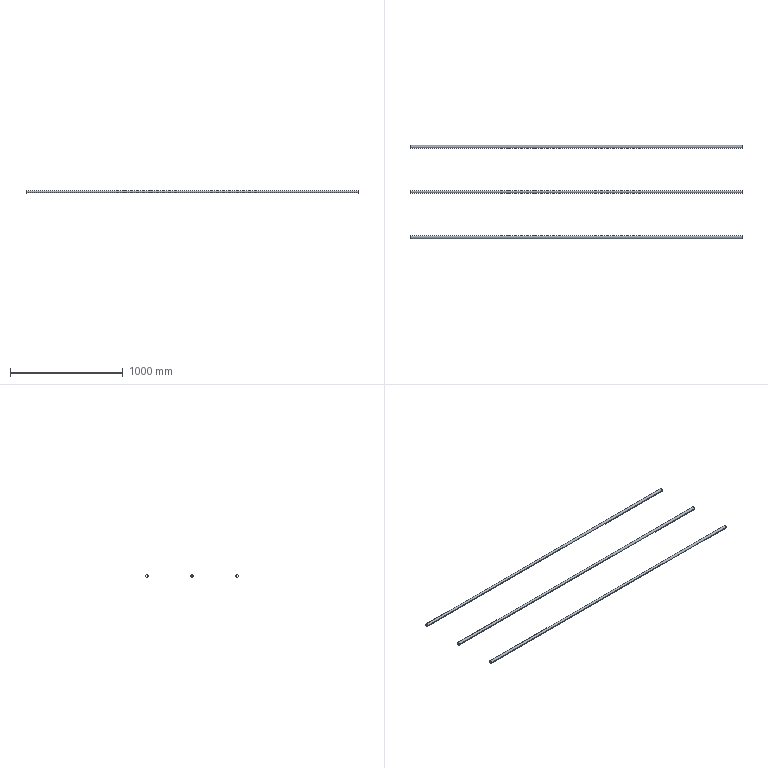Part | STEP file | E3-中转釜护栏1栏杆_Default<As Machined> | 3 solids | 18 faces | box 2940 x 825 x 25 mm | volume 976737 mm3 | cylinder 12 | plane 6 | commonest cylinder face diameters 22 x6 25 x6
STEP:
#1=CARTESIAN_POINT('',(0.,0.,0.));
#2=DIRECTION('',(0.,0.,1.));
#3=DIRECTION('',(1.,0.,0.));
#4=AXIS2_PLACEMENT_3D('',#1,#2,#3);
#5=CARTESIAN_POINT('',(1470.,787.5,0.));
#6=VERTEX_POINT('',#5);
#7=CARTESIAN_POINT('',(1470.,812.5,0.));
#8=VERTEX_POINT('',#7);
#9=CARTESIAN_POINT('',(1470.,800.,0.));
#10=DIRECTION('',(-1.,0.,0.));
#11=DIRECTION('',(0.,1.,0.));
#12=AXIS2_PLACEMENT_3D('',#9,#10,#11);
#13=CIRCLE('',#12,12.5);
#14=CARTESIAN_POINT('',(1470.,800.,0.));
#15=DIRECTION('',(-1.,0.,0.));
#16=DIRECTION('',(0.,-1.,0.));
#17=AXIS2_PLACEMENT_3D('',#14,#15,#16);
#18=CYLINDRICAL_SURFACE('',#17,12.5);
#19=CARTESIAN_POINT('',(-3.142,0.));
#20=DIRECTION('',(1.,0.));
#21=VECTOR('',#20,1.);
#22=LINE('',#19,#21);
#23=(GEOMETRIC_REPRESENTATION_CONTEXT(2)PARAMETRIC_REPRESENTATION_CONTEXT()REPRESENTATION_CONTEXT('',''));
#24=DEFINITIONAL_REPRESENTATION('',(#22),#23);
#25=PCURVE('',#18,#24);
#26=CARTESIAN_POINT('',(1470.,800.,0.));
#27=DIRECTION('',(1.,0.,0.));
#28=DIRECTION('',(0.,1.,0.));
#29=AXIS2_PLACEMENT_3D('',#26,#27,#28);
#30=PLANE('',#29);
#31=CARTESIAN_POINT('',(12.5,0.));
#32=CARTESIAN_POINT('',(12.5,-21.651));
#33=CARTESIAN_POINT('',(-6.25,-10.825));
#34=CARTESIAN_POINT('',(-25.,0.));
#35=CARTESIAN_POINT('',(-6.25,10.825));
#36=CARTESIAN_POINT('',(12.5,21.651));
#37=CARTESIAN_POINT('',(12.5,0.));
#38=(BOUNDED_CURVE()B_SPLINE_CURVE(2,(#31,#32,#33,#34,#35,#36,#37),.UNSPECIFIED.,.T.,.F.)B_SPLINE_CURVE_WITH_KNOTS((1,2,2,2,2,1),(-2.094,0.,2.094,4.189,6.283,8.378),.UNSPECIFIED.)CURVE()GEOMETRIC_REPRESENTATION_ITEM()RATIONAL_B_SPLINE_CURVE((1.,0.5,1.,0.5,1.,0.5,1.))REPRESENTATION_ITEM(''));
#39=(GEOMETRIC_REPRESENTATION_CONTEXT(2)PARAMETRIC_REPRESENTATION_CONTEXT()REPRESENTATION_CONTEXT('',''));
#40=DEFINITIONAL_REPRESENTATION('',(#38),#39);
#41=PCURVE('',#30,#40);
#42=SURFACE_CURVE('',#13,(#25,#41),.PCURVE_S1.);
#43=EDGE_CURVE('',#6,#8,#42,.T.);
#44=ORIENTED_EDGE('',*,*,#43,.T.);
#45=CARTESIAN_POINT('',(-1470.,812.5,0.));
#46=VERTEX_POINT('',#45);
#47=CARTESIAN_POINT('',(1470.,812.5,0.));
#48=DIRECTION('',(-1.,0.,0.));
#49=VECTOR('',#48,1.);
#50=LINE('',#47,#49);
#51=CARTESIAN_POINT('',(3.142,0.));
#52=DIRECTION('',(0.,1.));
#53=VECTOR('',#52,1.);
#54=LINE('',#51,#53);
#55=(GEOMETRIC_REPRESENTATION_CONTEXT(2)PARAMETRIC_REPRESENTATION_CONTEXT()REPRESENTATION_CONTEXT('',''));
#56=DEFINITIONAL_REPRESENTATION('',(#54),#55);
#57=PCURVE('',#18,#56);
#58=CARTESIAN_POINT('',(1470.,800.,0.));
#59=DIRECTION('',(-1.,0.,0.));
#60=DIRECTION('',(0.,-1.,0.));
#61=AXIS2_PLACEMENT_3D('',#58,#59,#60);
#62=CYLINDRICAL_SURFACE('',#61,12.5);
#63=CARTESIAN_POINT('',(3.142,0.));
#64=DIRECTION('',(0.,1.));
#65=VECTOR('',#64,1.);
#66=LINE('',#63,#65);
#67=(GEOMETRIC_REPRESENTATION_CONTEXT(2)PARAMETRIC_REPRESENTATION_CONTEXT()REPRESENTATION_CONTEXT('',''));
#68=DEFINITIONAL_REPRESENTATION('',(#66),#67);
#69=PCURVE('',#62,#68);
#70=SURFACE_CURVE('',#50,(#57,#69),.PCURVE_S1.);
#71=EDGE_CURVE('',#8,#46,#70,.T.);
#72=ORIENTED_EDGE('',*,*,#71,.T.);
#73=CARTESIAN_POINT('',(-1470.,787.5,0.));
#74=VERTEX_POINT('',#73);
#75=CARTESIAN_POINT('',(-1470.,800.,0.));
#76=DIRECTION('',(-1.,0.,0.));
#77=DIRECTION('',(0.,1.,0.));
#78=AXIS2_PLACEMENT_3D('',#75,#76,#77);
#79=CIRCLE('',#78,12.5);
#80=CARTESIAN_POINT('',(-3.142,2940.));
#81=DIRECTION('',(1.,0.));
#82=VECTOR('',#81,1.);
#83=LINE('',#80,#82);
#84=(GEOMETRIC_REPRESENTATION_CONTEXT(2)PARAMETRIC_REPRESENTATION_CONTEXT()REPRESENTATION_CONTEXT('',''));
#85=DEFINITIONAL_REPRESENTATION('',(#83),#84);
#86=PCURVE('',#18,#85);
#87=CARTESIAN_POINT('',(-1470.,800.,0.));
#88=DIRECTION('',(1.,0.,0.));
#89=DIRECTION('',(0.,1.,0.));
#90=AXIS2_PLACEMENT_3D('',#87,#88,#89);
#91=PLANE('',#90);
#92=CARTESIAN_POINT('',(12.5,0.));
#93=CARTESIAN_POINT('',(12.5,-21.651));
#94=CARTESIAN_POINT('',(-6.25,-10.825));
#95=CARTESIAN_POINT('',(-25.,0.));
#96=CARTESIAN_POINT('',(-6.25,10.825));
#97=CARTESIAN_POINT('',(12.5,21.651));
#98=CARTESIAN_POINT('',(12.5,0.));
#99=(BOUNDED_CURVE()B_SPLINE_CURVE(2,(#92,#93,#94,#95,#96,#97,#98),.UNSPECIFIED.,.T.,.F.)B_SPLINE_CURVE_WITH_KNOTS((1,2,2,2,2,1),(-2.094,0.,2.094,4.189,6.283,8.378),.UNSPECIFIED.)CURVE()GEOMETRIC_REPRESENTATION_ITEM()RATIONAL_B_SPLINE_CURVE((1.,0.5,1.,0.5,1.,0.5,1.))REPRESENTATION_ITEM(''));
#100=(GEOMETRIC_REPRESENTATION_CONTEXT(2)PARAMETRIC_REPRESENTATION_CONTEXT()REPRESENTATION_CONTEXT('',''));
#101=DEFINITIONAL_REPRESENTATION('',(#99),#100);
#102=PCURVE('',#91,#101);
#103=SURFACE_CURVE('',#79,(#86,#102),.PCURVE_S1.);
#104=EDGE_CURVE('',#74,#46,#103,.T.);
#105=ORIENTED_EDGE('',*,*,#104,.F.);
#106=CARTESIAN_POINT('',(1470.,787.5,0.));
#107=DIRECTION('',(-1.,0.,0.));
#108=VECTOR('',#107,1.);
#109=LINE('',#106,#108);
#110=CARTESIAN_POINT('',(0.,0.));
#111=DIRECTION('',(0.,1.));
#112=VECTOR('',#111,1.);
#113=LINE('',#110,#112);
#114=(GEOMETRIC_REPRESENTATION_CONTEXT(2)PARAMETRIC_REPRESENTATION_CONTEXT()REPRESENTATION_CONTEXT('',''));
#115=DEFINITIONAL_REPRESENTATION('',(#113),#114);
#116=PCURVE('',#18,#115);
#117=CARTESIAN_POINT('',(6.283,0.));
#118=DIRECTION('',(0.,1.));
#119=VECTOR('',#118,1.);
#120=LINE('',#117,#119);
#121=(GEOMETRIC_REPRESENTATION_CONTEXT(2)PARAMETRIC_REPRESENTATION_CONTEXT()REPRESENTATION_CONTEXT('',''));
#122=DEFINITIONAL_REPRESENTATION('',(#120),#121);
#123=PCURVE('',#62,#122);
#124=SURFACE_CURVE('',#109,(#116,#123),.PCURVE_S1.);
#125=EDGE_CURVE('',#6,#74,#124,.T.);
#126=ORIENTED_EDGE('',*,*,#125,.F.);
#127=EDGE_LOOP('',(#44,#72,#105,#126));
#128=FACE_BOUND('',#127,.T.);
#129=ADVANCED_FACE('',(#128),#18,.T.);
#130=CARTESIAN_POINT('',(1470.,789.,0.));
#131=VERTEX_POINT('',#130);
#132=CARTESIAN_POINT('',(-1470.,789.,0.));
#133=VERTEX_POINT('',#132);
#134=CARTESIAN_POINT('',(1470.,789.,0.));
#135=DIRECTION('',(-1.,0.,0.));
#136=VECTOR('',#135,1.);
#137=LINE('',#134,#136);
#138=CARTESIAN_POINT('',(1470.,800.,0.));
#139=DIRECTION('',(-1.,0.,0.));
#140=DIRECTION('',(0.,-1.,0.));
#141=AXIS2_PLACEMENT_3D('',#138,#139,#140);
#142=CYLINDRICAL_SURFACE('',#141,11.);
#143=CARTESIAN_POINT('',(6.283,0.));
#144=DIRECTION('',(0.,1.));
#145=VECTOR('',#144,1.);
#146=LINE('',#143,#145);
#147=(GEOMETRIC_REPRESENTATION_CONTEXT(2)PARAMETRIC_REPRESENTATION_CONTEXT()REPRESENTATION_CONTEXT('',''));
#148=DEFINITIONAL_REPRESENTATION('',(#146),#147);
#149=PCURVE('',#142,#148);
#150=CARTESIAN_POINT('',(1470.,800.,0.));
#151=DIRECTION('',(-1.,0.,0.));
#152=DIRECTION('',(0.,-1.,0.));
#153=AXIS2_PLACEMENT_3D('',#150,#151,#152);
#154=CYLINDRICAL_SURFACE('',#153,11.);
#155=CARTESIAN_POINT('',(0.,0.));
#156=DIRECTION('',(0.,1.));
#157=VECTOR('',#156,1.);
#158=LINE('',#155,#157);
#159=(GEOMETRIC_REPRESENTATION_CONTEXT(2)PARAMETRIC_REPRESENTATION_CONTEXT()REPRESENTATION_CONTEXT('',''));
#160=DEFINITIONAL_REPRESENTATION('',(#158),#159);
#161=PCURVE('',#154,#160);
#162=SURFACE_CURVE('',#137,(#149,#161),.PCURVE_S1.);
#163=EDGE_CURVE('',#131,#133,#162,.T.);
#164=ORIENTED_EDGE('',*,*,#163,.T.);
#165=CARTESIAN_POINT('',(-1470.,811.,0.));
#166=VERTEX_POINT('',#165);
#167=CARTESIAN_POINT('',(-1470.,800.,0.));
#168=DIRECTION('',(-1.,0.,0.));
#169=DIRECTION('',(0.,1.,0.));
#170=AXIS2_PLACEMENT_3D('',#167,#168,#169);
#171=CIRCLE('',#170,11.);
#172=CARTESIAN_POINT('',(3.142,2940.));
#173=DIRECTION('',(1.,0.));
#174=VECTOR('',#173,1.);
#175=LINE('',#172,#174);
#176=(GEOMETRIC_REPRESENTATION_CONTEXT(2)PARAMETRIC_REPRESENTATION_CONTEXT()REPRESENTATION_CONTEXT('',''));
#177=DEFINITIONAL_REPRESENTATION('',(#175),#176);
#178=PCURVE('',#142,#177);
#179=CARTESIAN_POINT('',(11.,0.));
#180=CARTESIAN_POINT('',(11.,-19.053));
#181=CARTESIAN_POINT('',(-5.5,-9.526));
#182=CARTESIAN_POINT('',(-22.,0.));
#183=CARTESIAN_POINT('',(-5.5,9.526));
#184=CARTESIAN_POINT('',(11.,19.053));
#185=CARTESIAN_POINT('',(11.,0.));
#186=(BOUNDED_CURVE()B_SPLINE_CURVE(2,(#179,#180,#181,#182,#183,#184,#185),.UNSPECIFIED.,.T.,.F.)B_SPLINE_CURVE_WITH_KNOTS((1,2,2,2,2,1),(-2.094,0.,2.094,4.189,6.283,8.378),.UNSPECIFIED.)CURVE()GEOMETRIC_REPRESENTATION_ITEM()RATIONAL_B_SPLINE_CURVE((1.,0.5,1.,0.5,1.,0.5,1.))REPRESENTATION_ITEM(''));
#187=(GEOMETRIC_REPRESENTATION_CONTEXT(2)PARAMETRIC_REPRESENTATION_CONTEXT()REPRESENTATION_CONTEXT('',''));
#188=DEFINITIONAL_REPRESENTATION('',(#186),#187);
#189=PCURVE('',#91,#188);
#190=SURFACE_CURVE('',#171,(#178,#189),.PCURVE_S1.);
#191=EDGE_CURVE('',#166,#133,#190,.T.);
#192=ORIENTED_EDGE('',*,*,#191,.F.);
#193=CARTESIAN_POINT('',(1470.,811.,0.));
#194=VERTEX_POINT('',#193);
#195=CARTESIAN_POINT('',(1470.,811.,0.));
#196=DIRECTION('',(-1.,0.,0.));
#197=VECTOR('',#196,1.);
#198=LINE('',#195,#197);
#199=CARTESIAN_POINT('',(3.142,0.));
#200=DIRECTION('',(0.,1.));
#201=VECTOR('',#200,1.);
#202=LINE('',#199,#201);
#203=(GEOMETRIC_REPRESENTATION_CONTEXT(2)PARAMETRIC_REPRESENTATION_CONTEXT()REPRESENTATION_CONTEXT('',''));
#204=DEFINITIONAL_REPRESENTATION('',(#202),#203);
#205=PCURVE('',#142,#204);
#206=CARTESIAN_POINT('',(3.142,0.));
#207=DIRECTION('',(0.,1.));
#208=VECTOR('',#207,1.);
#209=LINE('',#206,#208);
#210=(GEOMETRIC_REPRESENTATION_CONTEXT(2)PARAMETRIC_REPRESENTATION_CONTEXT()REPRESENTATION_CONTEXT('',''));
#211=DEFINITIONAL_REPRESENTATION('',(#209),#210);
#212=PCURVE('',#154,#211);
#213=SURFACE_CURVE('',#198,(#205,#212),.PCURVE_S1.);
#214=EDGE_CURVE('',#194,#166,#213,.T.);
#215=ORIENTED_EDGE('',*,*,#214,.F.);
#216=CARTESIAN_POINT('',(1470.,800.,0.));
#217=DIRECTION('',(-1.,0.,0.));
#218=DIRECTION('',(0.,1.,0.));
#219=AXIS2_PLACEMENT_3D('',#216,#217,#218);
#220=CIRCLE('',#219,11.);
#221=CARTESIAN_POINT('',(3.142,0.));
#222=DIRECTION('',(1.,0.));
#223=VECTOR('',#222,1.);
#224=LINE('',#221,#223);
#225=(GEOMETRIC_REPRESENTATION_CONTEXT(2)PARAMETRIC_REPRESENTATION_CONTEXT()REPRESENTATION_CONTEXT('',''));
#226=DEFINITIONAL_REPRESENTATION('',(#224),#225);
#227=PCURVE('',#142,#226);
#228=CARTESIAN_POINT('',(11.,0.));
#229=CARTESIAN_POINT('',(11.,-19.053));
#230=CARTESIAN_POINT('',(-5.5,-9.526));
#231=CARTESIAN_POINT('',(-22.,0.));
#232=CARTESIAN_POINT('',(-5.5,9.526));
#233=CARTESIAN_POINT('',(11.,19.053));
#234=CARTESIAN_POINT('',(11.,0.));
#235=(BOUNDED_CURVE()B_SPLINE_CURVE(2,(#228,#229,#230,#231,#232,#233,#234),.UNSPECIFIED.,.T.,.F.)B_SPLINE_CURVE_WITH_KNOTS((1,2,2,2,2,1),(-2.094,0.,2.094,4.189,6.283,8.378),.UNSPECIFIED.)CURVE()GEOMETRIC_REPRESENTATION_ITEM()RATIONAL_B_SPLINE_CURVE((1.,0.5,1.,0.5,1.,0.5,1.))REPRESENTATION_ITEM(''));
#236=(GEOMETRIC_REPRESENTATION_CONTEXT(2)PARAMETRIC_REPRESENTATION_CONTEXT()REPRESENTATION_CONTEXT('',''));
#237=DEFINITIONAL_REPRESENTATION('',(#235),#236);
#238=PCURVE('',#30,#237);
#239=SURFACE_CURVE('',#220,(#227,#238),.PCURVE_S1.);
#240=EDGE_CURVE('',#194,#131,#239,.T.);
#241=ORIENTED_EDGE('',*,*,#240,.T.);
#242=EDGE_LOOP('',(#164,#192,#215,#241));
#243=FACE_BOUND('',#242,.F.);
#244=ADVANCED_FACE('',(#243),#142,.F.);
#245=CARTESIAN_POINT('',(-1470.,800.,0.));
#246=DIRECTION('',(-1.,0.,0.));
#247=DIRECTION('',(0.,1.,0.));
#248=AXIS2_PLACEMENT_3D('',#245,#246,#247);
#249=CIRCLE('',#248,11.);
#250=CARTESIAN_POINT('',(-3.142,2940.));
#251=DIRECTION('',(1.,0.));
#252=VECTOR('',#251,1.);
#253=LINE('',#250,#252);
#254=(GEOMETRIC_REPRESENTATION_CONTEXT(2)PARAMETRIC_REPRESENTATION_CONTEXT()REPRESENTATION_CONTEXT('',''));
#255=DEFINITIONAL_REPRESENTATION('',(#253),#254);
#256=PCURVE('',#154,#255);
#257=CARTESIAN_POINT('',(11.,0.));
#258=CARTESIAN_POINT('',(11.,-19.053));
#259=CARTESIAN_POINT('',(-5.5,-9.526));
#260=CARTESIAN_POINT('',(-22.,0.));
#261=CARTESIAN_POINT('',(-5.5,9.526));
#262=CARTESIAN_POINT('',(11.,19.053));
#263=CARTESIAN_POINT('',(11.,0.));
#264=(BOUNDED_CURVE()B_SPLINE_CURVE(2,(#257,#258,#259,#260,#261,#262,#263),.UNSPECIFIED.,.T.,.F.)B_SPLINE_CURVE_WITH_KNOTS((1,2,2,2,2,1),(-2.094,0.,2.094,4.189,6.283,8.378),.UNSPECIFIED.)CURVE()GEOMETRIC_REPRESENTATION_ITEM()RATIONAL_B_SPLINE_CURVE((1.,0.5,1.,0.5,1.,0.5,1.))REPRESENTATION_ITEM(''));
#265=(GEOMETRIC_REPRESENTATION_CONTEXT(2)PARAMETRIC_REPRESENTATION_CONTEXT()REPRESENTATION_CONTEXT('',''));
#266=DEFINITIONAL_REPRESENTATION('',(#264),#265);
#267=PCURVE('',#91,#266);
#268=SURFACE_CURVE('',#249,(#256,#267),.PCURVE_S1.);
#269=EDGE_CURVE('',#133,#166,#268,.T.);
#270=ORIENTED_EDGE('',*,*,#269,.F.);
#271=ORIENTED_EDGE('',*,*,#163,.F.);
#272=CARTESIAN_POINT('',(1470.,800.,0.));
#273=DIRECTION('',(-1.,0.,0.));
#274=DIRECTION('',(0.,1.,0.));
#275=AXIS2_PLACEMENT_3D('',#272,#273,#274);
#276=CIRCLE('',#275,11.);
#277=CARTESIAN_POINT('',(-3.142,0.));
#278=DIRECTION('',(1.,0.));
#279=VECTOR('',#278,1.);
#280=LINE('',#277,#279);
#281=(GEOMETRIC_REPRESENTATION_CONTEXT(2)PARAMETRIC_REPRESENTATION_CONTEXT()REPRESENTATION_CONTEXT('',''));
#282=DEFINITIONAL_REPRESENTATION('',(#280),#281);
#283=PCURVE('',#154,#282);
#284=CARTESIAN_POINT('',(11.,0.));
#285=CARTESIAN_POINT('',(11.,-19.053));
#286=CARTESIAN_POINT('',(-5.5,-9.526));
#287=CARTESIAN_POINT('',(-22.,0.));
#288=CARTESIAN_POINT('',(-5.5,9.526));
#289=CARTESIAN_POINT('',(11.,19.053));
#290=CARTESIAN_POINT('',(11.,0.));
#291=(BOUNDED_CURVE()B_SPLINE_CURVE(2,(#284,#285,#286,#287,#288,#289,#290),.UNSPECIFIED.,.T.,.F.)B_SPLINE_CURVE_WITH_KNOTS((1,2,2,2,2,1),(-2.094,0.,2.094,4.189,6.283,8.378),.UNSPECIFIED.)CURVE()GEOMETRIC_REPRESENTATION_ITEM()RATIONAL_B_SPLINE_CURVE((1.,0.5,1.,0.5,1.,0.5,1.))REPRESENTATION_ITEM(''));
#292=(GEOMETRIC_REPRESENTATION_CONTEXT(2)PARAMETRIC_REPRESENTATION_CONTEXT()REPRESENTATION_CONTEXT('',''));
#293=DEFINITIONAL_REPRESENTATION('',(#291),#292);
#294=PCURVE('',#30,#293);
#295=SURFACE_CURVE('',#276,(#283,#294),.PCURVE_S1.);
#296=EDGE_CURVE('',#131,#194,#295,.T.);
#297=ORIENTED_EDGE('',*,*,#296,.T.);
#298=ORIENTED_EDGE('',*,*,#214,.T.);
#299=EDGE_LOOP('',(#270,#271,#297,#298));
#300=FACE_BOUND('',#299,.F.);
#301=ADVANCED_FACE('',(#300),#154,.F.);
#302=ORIENTED_EDGE('',*,*,#71,.F.);
#303=CARTESIAN_POINT('',(1470.,800.,0.));
#304=DIRECTION('',(-1.,0.,0.));
#305=DIRECTION('',(0.,1.,0.));
#306=AXIS2_PLACEMENT_3D('',#303,#304,#305);
#307=CIRCLE('',#306,12.5);
#308=CARTESIAN_POINT('',(3.142,0.));
#309=DIRECTION('',(1.,0.));
#310=VECTOR('',#309,1.);
#311=LINE('',#308,#310);
#312=(GEOMETRIC_REPRESENTATION_CONTEXT(2)PARAMETRIC_REPRESENTATION_CONTEXT()REPRESENTATION_CONTEXT('',''));
#313=DEFINITIONAL_REPRESENTATION('',(#311),#312);
#314=PCURVE('',#62,#313);
#315=CARTESIAN_POINT('',(12.5,0.));
#316=CARTESIAN_POINT('',(12.5,-21.651));
#317=CARTESIAN_POINT('',(-6.25,-10.825));
#318=CARTESIAN_POINT('',(-25.,0.));
#319=CARTESIAN_POINT('',(-6.25,10.825));
#320=CARTESIAN_POINT('',(12.5,21.651));
#321=CARTESIAN_POINT('',(12.5,0.));
#322=(BOUNDED_CURVE()B_SPLINE_CURVE(2,(#315,#316,#317,#318,#319,#320,#321),.UNSPECIFIED.,.T.,.F.)B_SPLINE_CURVE_WITH_KNOTS((1,2,2,2,2,1),(-2.094,0.,2.094,4.189,6.283,8.378),.UNSPECIFIED.)CURVE()GEOMETRIC_REPRESENTATION_ITEM()RATIONAL_B_SPLINE_CURVE((1.,0.5,1.,0.5,1.,0.5,1.))REPRESENTATION_ITEM(''));
#323=(GEOMETRIC_REPRESENTATION_CONTEXT(2)PARAMETRIC_REPRESENTATION_CONTEXT()REPRESENTATION_CONTEXT('',''));
#324=DEFINITIONAL_REPRESENTATION('',(#322),#323);
#325=PCURVE('',#30,#324);
#326=SURFACE_CURVE('',#307,(#314,#325),.PCURVE_S1.);
#327=EDGE_CURVE('',#8,#6,#326,.T.);
#328=ORIENTED_EDGE('',*,*,#327,.T.);
#329=ORIENTED_EDGE('',*,*,#125,.T.);
#330=CARTESIAN_POINT('',(-1470.,800.,0.));
#331=DIRECTION('',(-1.,0.,0.));
#332=DIRECTION('',(0.,1.,0.));
#333=AXIS2_PLACEMENT_3D('',#330,#331,#332);
#334=CIRCLE('',#333,12.5);
#335=CARTESIAN_POINT('',(3.142,2940.));
#336=DIRECTION('',(1.,0.));
#337=VECTOR('',#336,1.);
#338=LINE('',#335,#337);
#339=(GEOMETRIC_REPRESENTATION_CONTEXT(2)PARAMETRIC_REPRESENTATION_CONTEXT()REPRESENTATION_CONTEXT('',''));
#340=DEFINITIONAL_REPRESENTATION('',(#338),#339);
#341=PCURVE('',#62,#340);
#342=CARTESIAN_POINT('',(12.5,0.));
#343=CARTESIAN_POINT('',(12.5,-21.651));
#344=CARTESIAN_POINT('',(-6.25,-10.825));
#345=CARTESIAN_POINT('',(-25.,0.));
#346=CARTESIAN_POINT('',(-6.25,10.825));
#347=CARTESIAN_POINT('',(12.5,21.651));
#348=CARTESIAN_POINT('',(12.5,0.));
#349=(BOUNDED_CURVE()B_SPLINE_CURVE(2,(#342,#343,#344,#345,#346,#347,#348),.UNSPECIFIED.,.T.,.F.)B_SPLINE_CURVE_WITH_KNOTS((1,2,2,2,2,1),(-2.094,0.,2.094,4.189,6.283,8.378),.UNSPECIFIED.)CURVE()GEOMETRIC_REPRESENTATION_ITEM()RATIONAL_B_SPLINE_CURVE((1.,0.5,1.,0.5,1.,0.5,1.))REPRESENTATION_ITEM(''));
#350=(GEOMETRIC_REPRESENTATION_CONTEXT(2)PARAMETRIC_REPRESENTATION_CONTEXT()REPRESENTATION_CONTEXT('',''));
#351=DEFINITIONAL_REPRESENTATION('',(#349),#350);
#352=PCURVE('',#91,#351);
#353=SURFACE_CURVE('',#334,(#341,#352),.PCURVE_S1.);
#354=EDGE_CURVE('',#46,#74,#353,.T.);
#355=ORIENTED_EDGE('',*,*,#354,.F.);
#356=EDGE_LOOP('',(#302,#328,#329,#355));
#357=FACE_BOUND('',#356,.T.);
#358=ADVANCED_FACE('',(#357),#62,.T.);
#359=ORIENTED_EDGE('',*,*,#296,.T.);
#360=ORIENTED_EDGE('',*,*,#240,.T.);
#361=EDGE_LOOP('',(#359,#360));
#362=FACE_BOUND('',#361,.T.);
#363=ORIENTED_EDGE('',*,*,#43,.F.);
#364=ORIENTED_EDGE('',*,*,#327,.F.);
#365=EDGE_LOOP('',(#363,#364));
#366=FACE_BOUND('',#365,.T.);
#367=ADVANCED_FACE('',(#362,#366),#30,.T.);
#368=ORIENTED_EDGE('',*,*,#269,.F.);
#369=ORIENTED_EDGE('',*,*,#191,.F.);
#370=EDGE_LOOP('',(#368,#369));
#371=FACE_BOUND('',#370,.T.);
#372=ORIENTED_EDGE('',*,*,#104,.T.);
#373=ORIENTED_EDGE('',*,*,#354,.T.);
#374=EDGE_LOOP('',(#372,#373));
#375=FACE_BOUND('',#374,.T.);
#376=ADVANCED_FACE('',(#371,#375),#91,.F.);
#377=CLOSED_SHELL('',(#129,#244,#301,#358,#367,#376));
#378=MANIFOLD_SOLID_BREP('',#377);
#379=CARTESIAN_POINT('',(1470.,-12.5,0.));
#380=VERTEX_POINT('',#379);
#381=CARTESIAN_POINT('',(1470.,12.5,0.));
#382=VERTEX_POINT('',#381);
#383=CARTESIAN_POINT('',(1470.,0.,0.));
#384=DIRECTION('',(-1.,0.,0.));
#385=DIRECTION('',(0.,1.,0.));
#386=AXIS2_PLACEMENT_3D('',#383,#384,#385);
#387=CIRCLE('',#386,12.5);
#388=CARTESIAN_POINT('',(1470.,0.,0.));
#389=DIRECTION('',(-1.,0.,0.));
#390=DIRECTION('',(0.,-1.,0.));
#391=AXIS2_PLACEMENT_3D('',#388,#389,#390);
#392=CYLINDRICAL_SURFACE('',#391,12.5);
#393=CARTESIAN_POINT('',(-3.142,0.));
#394=DIRECTION('',(1.,0.));
#395=VECTOR('',#394,1.);
#396=LINE('',#393,#395);
#397=(GEOMETRIC_REPRESENTATION_CONTEXT(2)PARAMETRIC_REPRESENTATION_CONTEXT()REPRESENTATION_CONTEXT('',''));
#398=DEFINITIONAL_REPRESENTATION('',(#396),#397);
#399=PCURVE('',#392,#398);
#400=CARTESIAN_POINT('',(1470.,0.,0.));
#401=DIRECTION('',(1.,0.,0.));
#402=DIRECTION('',(0.,1.,0.));
#403=AXIS2_PLACEMENT_3D('',#400,#401,#402);
#404=PLANE('',#403);
#405=CARTESIAN_POINT('',(12.5,0.));
#406=CARTESIAN_POINT('',(12.5,-21.651));
#407=CARTESIAN_POINT('',(-6.25,-10.825));
#408=CARTESIAN_POINT('',(-25.,0.));
#409=CARTESIAN_POINT('',(-6.25,10.825));
#410=CARTESIAN_POINT('',(12.5,21.651));
#411=CARTESIAN_POINT('',(12.5,0.));
#412=(BOUNDED_CURVE()B_SPLINE_CURVE(2,(#405,#406,#407,#408,#409,#410,#411),.UNSPECIFIED.,.T.,.F.)B_SPLINE_CURVE_WITH_KNOTS((1,2,2,2,2,1),(-2.094,0.,2.094,4.189,6.283,8.378),.UNSPECIFIED.)CURVE()GEOMETRIC_REPRESENTATION_ITEM()RATIONAL_B_SPLINE_CURVE((1.,0.5,1.,0.5,1.,0.5,1.))REPRESENTATION_ITEM(''));
#413=(GEOMETRIC_REPRESENTATION_CONTEXT(2)PARAMETRIC_REPRESENTATION_CONTEXT()REPRESENTATION_CONTEXT('',''));
#414=DEFINITIONAL_REPRESENTATION('',(#412),#413);
#415=PCURVE('',#404,#414);
#416=SURFACE_CURVE('',#387,(#399,#415),.PCURVE_S1.);
#417=EDGE_CURVE('',#380,#382,#416,.T.);
#418=ORIENTED_EDGE('',*,*,#417,.T.);
#419=CARTESIAN_POINT('',(-1470.,12.5,0.));
#420=VERTEX_POINT('',#419);
#421=CARTESIAN_POINT('',(1470.,12.5,0.));
#422=DIRECTION('',(-1.,0.,0.));
#423=VECTOR('',#422,1.);
#424=LINE('',#421,#423);
#425=CARTESIAN_POINT('',(3.142,0.));
#426=DIRECTION('',(0.,1.));
#427=VECTOR('',#426,1.);
#428=LINE('',#425,#427);
#429=(GEOMETRIC_REPRESENTATION_CONTEXT(2)PARAMETRIC_REPRESENTATION_CONTEXT()REPRESENTATION_CONTEXT('',''));
#430=DEFINITIONAL_REPRESENTATION('',(#428),#429);
#431=PCURVE('',#392,#430);
#432=CARTESIAN_POINT('',(1470.,0.,0.));
#433=DIRECTION('',(-1.,0.,0.));
#434=DIRECTION('',(0.,-1.,0.));
#435=AXIS2_PLACEMENT_3D('',#432,#433,#434);
#436=CYLINDRICAL_SURFACE('',#435,12.5);
#437=CARTESIAN_POINT('',(3.142,0.));
#438=DIRECTION('',(0.,1.));
#439=VECTOR('',#438,1.);
#440=LINE('',#437,#439);
#441=(GEOMETRIC_REPRESENTATION_CONTEXT(2)PARAMETRIC_REPRESENTATION_CONTEXT()REPRESENTATION_CONTEXT('',''));
#442=DEFINITIONAL_REPRESENTATION('',(#440),#441);
#443=PCURVE('',#436,#442);
#444=SURFACE_CURVE('',#424,(#431,#443),.PCURVE_S1.);
#445=EDGE_CURVE('',#382,#420,#444,.T.);
#446=ORIENTED_EDGE('',*,*,#445,.T.);
#447=CARTESIAN_POINT('',(-1470.,-12.5,0.));
#448=VERTEX_POINT('',#447);
#449=CARTESIAN_POINT('',(-1470.,0.,0.));
#450=DIRECTION('',(-1.,0.,0.));
#451=DIRECTION('',(0.,1.,0.));
#452=AXIS2_PLACEMENT_3D('',#449,#450,#451);
#453=CIRCLE('',#452,12.5);
#454=CARTESIAN_POINT('',(-3.142,2940.));
#455=DIRECTION('',(1.,0.));
#456=VECTOR('',#455,1.);
#457=LINE('',#454,#456);
#458=(GEOMETRIC_REPRESENTATION_CONTEXT(2)PARAMETRIC_REPRESENTATION_CONTEXT()REPRESENTATION_CONTEXT('',''));
#459=DEFINITIONAL_REPRESENTATION('',(#457),#458);
#460=PCURVE('',#392,#459);
#461=CARTESIAN_POINT('',(-1470.,0.,0.));
#462=DIRECTION('',(1.,0.,0.));
#463=DIRECTION('',(0.,1.,0.));
#464=AXIS2_PLACEMENT_3D('',#461,#462,#463);
#465=PLANE('',#464);
#466=CARTESIAN_POINT('',(12.5,0.));
#467=CARTESIAN_POINT('',(12.5,-21.651));
#468=CARTESIAN_POINT('',(-6.25,-10.825));
#469=CARTESIAN_POINT('',(-25.,0.));
#470=CARTESIAN_POINT('',(-6.25,10.825));
#471=CARTESIAN_POINT('',(12.5,21.651));
#472=CARTESIAN_POINT('',(12.5,0.));
#473=(BOUNDED_CURVE()B_SPLINE_CURVE(2,(#466,#467,#468,#469,#470,#471,#472),.UNSPECIFIED.,.T.,.F.)B_SPLINE_CURVE_WITH_KNOTS((1,2,2,2,2,1),(-2.094,0.,2.094,4.189,6.283,8.378),.UNSPECIFIED.)CURVE()GEOMETRIC_REPRESENTATION_ITEM()RATIONAL_B_SPLINE_CURVE((1.,0.5,1.,0.5,1.,0.5,1.))REPRESENTATION_ITEM(''));
#474=(GEOMETRIC_REPRESENTATION_CONTEXT(2)PARAMETRIC_REPRESENTATION_CONTEXT()REPRESENTATION_CONTEXT('',''));
#475=DEFINITIONAL_REPRESENTATION('',(#473),#474);
#476=PCURVE('',#465,#475);
#477=SURFACE_CURVE('',#453,(#460,#476),.PCURVE_S1.);
#478=EDGE_CURVE('',#448,#420,#477,.T.);
#479=ORIENTED_EDGE('',*,*,#478,.F.);
#480=CARTESIAN_POINT('',(1470.,-12.5,0.));
#481=DIRECTION('',(-1.,0.,0.));
#482=VECTOR('',#481,1.);
#483=LINE('',#480,#482);
#484=CARTESIAN_POINT('',(0.,0.));
#485=DIRECTION('',(0.,1.));
#486=VECTOR('',#485,1.);
#487=LINE('',#484,#486);
#488=(GEOMETRIC_REPRESENTATION_CONTEXT(2)PARAMETRIC_REPRESENTATION_CONTEXT()REPRESENTATION_CONTEXT('',''));
#489=DEFINITIONAL_REPRESENTATION('',(#487),#488);
#490=PCURVE('',#392,#489);
#491=CARTESIAN_POINT('',(6.283,0.));
#492=DIRECTION('',(0.,1.));
#493=VECTOR('',#492,1.);
#494=LINE('',#491,#493);
#495=(GEOMETRIC_REPRESENTATION_CONTEXT(2)PARAMETRIC_REPRESENTATION_CONTEXT()REPRESENTATION_CONTEXT('',''));
#496=DEFINITIONAL_REPRESENTATION('',(#494),#495);
#497=PCURVE('',#436,#496);
#498=SURFACE_CURVE('',#483,(#490,#497),.PCURVE_S1.);
#499=EDGE_CURVE('',#380,#448,#498,.T.);
#500=ORIENTED_EDGE('',*,*,#499,.F.);
#501=EDGE_LOOP('',(#418,#446,#479,#500));
#502=FACE_BOUND('',#501,.T.);
#503=ADVANCED_FACE('',(#502),#392,.T.);
#504=CARTESIAN_POINT('',(1470.,-11.,0.));
#505=VERTEX_POINT('',#504);
#506=CARTESIAN_POINT('',(-1470.,-11.,0.));
#507=VERTEX_POINT('',#506);
#508=CARTESIAN_POINT('',(1470.,-11.,0.));
#509=DIRECTION('',(-1.,0.,0.));
#510=VECTOR('',#509,1.);
#511=LINE('',#508,#510);
#512=CARTESIAN_POINT('',(1470.,0.,0.));
#513=DIRECTION('',(-1.,0.,0.));
#514=DIRECTION('',(0.,-1.,0.));
#515=AXIS2_PLACEMENT_3D('',#512,#513,#514);
#516=CYLINDRICAL_SURFACE('',#515,11.);
#517=CARTESIAN_POINT('',(6.283,0.));
#518=DIRECTION('',(0.,1.));
#519=VECTOR('',#518,1.);
#520=LINE('',#517,#519);
#521=(GEOMETRIC_REPRESENTATION_CONTEXT(2)PARAMETRIC_REPRESENTATION_CONTEXT()REPRESENTATION_CONTEXT('',''));
#522=DEFINITIONAL_REPRESENTATION('',(#520),#521);
#523=PCURVE('',#516,#522);
#524=CARTESIAN_POINT('',(1470.,0.,0.));
#525=DIRECTION('',(-1.,0.,0.));
#526=DIRECTION('',(0.,-1.,0.));
#527=AXIS2_PLACEMENT_3D('',#524,#525,#526);
#528=CYLINDRICAL_SURFACE('',#527,11.);
#529=CARTESIAN_POINT('',(0.,0.));
#530=DIRECTION('',(0.,1.));
#531=VECTOR('',#530,1.);
#532=LINE('',#529,#531);
#533=(GEOMETRIC_REPRESENTATION_CONTEXT(2)PARAMETRIC_REPRESENTATION_CONTEXT()REPRESENTATION_CONTEXT('',''));
#534=DEFINITIONAL_REPRESENTATION('',(#532),#533);
#535=PCURVE('',#528,#534);
#536=SURFACE_CURVE('',#511,(#523,#535),.PCURVE_S1.);
#537=EDGE_CURVE('',#505,#507,#536,.T.);
#538=ORIENTED_EDGE('',*,*,#537,.T.);
#539=CARTESIAN_POINT('',(-1470.,11.,0.));
#540=VERTEX_POINT('',#539);
#541=CARTESIAN_POINT('',(-1470.,0.,0.));
#542=DIRECTION('',(-1.,0.,0.));
#543=DIRECTION('',(0.,1.,0.));
#544=AXIS2_PLACEMENT_3D('',#541,#542,#543);
#545=CIRCLE('',#544,11.);
#546=CARTESIAN_POINT('',(3.142,2940.));
#547=DIRECTION('',(1.,0.));
#548=VECTOR('',#547,1.);
#549=LINE('',#546,#548);
#550=(GEOMETRIC_REPRESENTATION_CONTEXT(2)PARAMETRIC_REPRESENTATION_CONTEXT()REPRESENTATION_CONTEXT('',''));
#551=DEFINITIONAL_REPRESENTATION('',(#549),#550);
#552=PCURVE('',#516,#551);
#553=CARTESIAN_POINT('',(11.,0.));
#554=CARTESIAN_POINT('',(11.,-19.053));
#555=CARTESIAN_POINT('',(-5.5,-9.526));
#556=CARTESIAN_POINT('',(-22.,0.));
#557=CARTESIAN_POINT('',(-5.5,9.526));
#558=CARTESIAN_POINT('',(11.,19.053));
#559=CARTESIAN_POINT('',(11.,0.));
#560=(BOUNDED_CURVE()B_SPLINE_CURVE(2,(#553,#554,#555,#556,#557,#558,#559),.UNSPECIFIED.,.T.,.F.)B_SPLINE_CURVE_WITH_KNOTS((1,2,2,2,2,1),(-2.094,0.,2.094,4.189,6.283,8.378),.UNSPECIFIED.)CURVE()GEOMETRIC_REPRESENTATION_ITEM()RATIONAL_B_SPLINE_CURVE((1.,0.5,1.,0.5,1.,0.5,1.))REPRESENTATION_ITEM(''));
#561=(GEOMETRIC_REPRESENTATION_CONTEXT(2)PARAMETRIC_REPRESENTATION_CONTEXT()REPRESENTATION_CONTEXT('',''));
#562=DEFINITIONAL_REPRESENTATION('',(#560),#561);
#563=PCURVE('',#465,#562);
#564=SURFACE_CURVE('',#545,(#552,#563),.PCURVE_S1.);
#565=EDGE_CURVE('',#540,#507,#564,.T.);
#566=ORIENTED_EDGE('',*,*,#565,.F.);
#567=CARTESIAN_POINT('',(1470.,11.,0.));
#568=VERTEX_POINT('',#567);
#569=CARTESIAN_POINT('',(1470.,11.,0.));
#570=DIRECTION('',(-1.,0.,0.));
#571=VECTOR('',#570,1.);
#572=LINE('',#569,#571);
#573=CARTESIAN_POINT('',(3.142,0.));
#574=DIRECTION('',(0.,1.));
#575=VECTOR('',#574,1.);
#576=LINE('',#573,#575);
#577=(GEOMETRIC_REPRESENTATION_CONTEXT(2)PARAMETRIC_REPRESENTATION_CONTEXT()REPRESENTATION_CONTEXT('',''));
#578=DEFINITIONAL_REPRESENTATION('',(#576),#577);
#579=PCURVE('',#516,#578);
#580=CARTESIAN_POINT('',(3.142,0.));
#581=DIRECTION('',(0.,1.));
#582=VECTOR('',#581,1.);
#583=LINE('',#580,#582);
#584=(GEOMETRIC_REPRESENTATION_CONTEXT(2)PARAMETRIC_REPRESENTATION_CONTEXT()REPRESENTATION_CONTEXT('',''));
#585=DEFINITIONAL_REPRESENTATION('',(#583),#584);
#586=PCURVE('',#528,#585);
#587=SURFACE_CURVE('',#572,(#579,#586),.PCURVE_S1.);
#588=EDGE_CURVE('',#568,#540,#587,.T.);
#589=ORIENTED_EDGE('',*,*,#588,.F.);
#590=CARTESIAN_POINT('',(1470.,0.,0.));
#591=DIRECTION('',(-1.,0.,0.));
#592=DIRECTION('',(0.,1.,0.));
#593=AXIS2_PLACEMENT_3D('',#590,#591,#592);
#594=CIRCLE('',#593,11.);
#595=CARTESIAN_POINT('',(3.142,0.));
#596=DIRECTION('',(1.,0.));
#597=VECTOR('',#596,1.);
#598=LINE('',#595,#597);
#599=(GEOMETRIC_REPRESENTATION_CONTEXT(2)PARAMETRIC_REPRESENTATION_CONTEXT()REPRESENTATION_CONTEXT('',''));
#600=DEFINITIONAL_REPRESENTATION('',(#598),#599);
#601=PCURVE('',#516,#600);
#602=CARTESIAN_POINT('',(11.,0.));
#603=CARTESIAN_POINT('',(11.,-19.053));
#604=CARTESIAN_POINT('',(-5.5,-9.526));
#605=CARTESIAN_POINT('',(-22.,0.));
#606=CARTESIAN_POINT('',(-5.5,9.526));
#607=CARTESIAN_POINT('',(11.,19.053));
#608=CARTESIAN_POINT('',(11.,0.));
#609=(BOUNDED_CURVE()B_SPLINE_CURVE(2,(#602,#603,#604,#605,#606,#607,#608),.UNSPECIFIED.,.T.,.F.)B_SPLINE_CURVE_WITH_KNOTS((1,2,2,2,2,1),(-2.094,0.,2.094,4.189,6.283,8.378),.UNSPECIFIED.)CURVE()GEOMETRIC_REPRESENTATION_ITEM()RATIONAL_B_SPLINE_CURVE((1.,0.5,1.,0.5,1.,0.5,1.))REPRESENTATION_ITEM(''));
#610=(GEOMETRIC_REPRESENTATION_CONTEXT(2)PARAMETRIC_REPRESENTATION_CONTEXT()REPRESENTATION_CONTEXT('',''));
#611=DEFINITIONAL_REPRESENTATION('',(#609),#610);
#612=PCURVE('',#404,#611);
#613=SURFACE_CURVE('',#594,(#601,#612),.PCURVE_S1.);
#614=EDGE_CURVE('',#568,#505,#613,.T.);
#615=ORIENTED_EDGE('',*,*,#614,.T.);
#616=EDGE_LOOP('',(#538,#566,#589,#615));
#617=FACE_BOUND('',#616,.F.);
#618=ADVANCED_FACE('',(#617),#516,.F.);
#619=CARTESIAN_POINT('',(-1470.,0.,0.));
#620=DIRECTION('',(-1.,0.,0.));
#621=DIRECTION('',(0.,1.,0.));
#622=AXIS2_PLACEMENT_3D('',#619,#620,#621);
#623=CIRCLE('',#622,11.);
#624=CARTESIAN_POINT('',(-3.142,2940.));
#625=DIRECTION('',(1.,0.));
#626=VECTOR('',#625,1.);
#627=LINE('',#624,#626);
#628=(GEOMETRIC_REPRESENTATION_CONTEXT(2)PARAMETRIC_REPRESENTATION_CONTEXT()REPRESENTATION_CONTEXT('',''));
#629=DEFINITIONAL_REPRESENTATION('',(#627),#628);
#630=PCURVE('',#528,#629);
#631=CARTESIAN_POINT('',(11.,0.));
#632=CARTESIAN_POINT('',(11.,-19.053));
#633=CARTESIAN_POINT('',(-5.5,-9.526));
#634=CARTESIAN_POINT('',(-22.,0.));
#635=CARTESIAN_POINT('',(-5.5,9.526));
#636=CARTESIAN_POINT('',(11.,19.053));
#637=CARTESIAN_POINT('',(11.,0.));
#638=(BOUNDED_CURVE()B_SPLINE_CURVE(2,(#631,#632,#633,#634,#635,#636,#637),.UNSPECIFIED.,.T.,.F.)B_SPLINE_CURVE_WITH_KNOTS((1,2,2,2,2,1),(-2.094,0.,2.094,4.189,6.283,8.378),.UNSPECIFIED.)CURVE()GEOMETRIC_REPRESENTATION_ITEM()RATIONAL_B_SPLINE_CURVE((1.,0.5,1.,0.5,1.,0.5,1.))REPRESENTATION_ITEM(''));
#639=(GEOMETRIC_REPRESENTATION_CONTEXT(2)PARAMETRIC_REPRESENTATION_CONTEXT()REPRESENTATION_CONTEXT('',''));
#640=DEFINITIONAL_REPRESENTATION('',(#638),#639);
#641=PCURVE('',#465,#640);
#642=SURFACE_CURVE('',#623,(#630,#641),.PCURVE_S1.);
#643=EDGE_CURVE('',#507,#540,#642,.T.);
#644=ORIENTED_EDGE('',*,*,#643,.F.);
#645=ORIENTED_EDGE('',*,*,#537,.F.);
#646=CARTESIAN_POINT('',(1470.,0.,0.));
#647=DIRECTION('',(-1.,0.,0.));
#648=DIRECTION('',(0.,1.,0.));
#649=AXIS2_PLACEMENT_3D('',#646,#647,#648);
#650=CIRCLE('',#649,11.);
#651=CARTESIAN_POINT('',(-3.142,0.));
#652=DIRECTION('',(1.,0.));
#653=VECTOR('',#652,1.);
#654=LINE('',#651,#653);
#655=(GEOMETRIC_REPRESENTATION_CONTEXT(2)PARAMETRIC_REPRESENTATION_CONTEXT()REPRESENTATION_CONTEXT('',''));
#656=DEFINITIONAL_REPRESENTATION('',(#654),#655);
#657=PCURVE('',#528,#656);
#658=CARTESIAN_POINT('',(11.,0.));
#659=CARTESIAN_POINT('',(11.,-19.053));
#660=CARTESIAN_POINT('',(-5.5,-9.526));
#661=CARTESIAN_POINT('',(-22.,0.));
#662=CARTESIAN_POINT('',(-5.5,9.526));
#663=CARTESIAN_POINT('',(11.,19.053));
#664=CARTESIAN_POINT('',(11.,0.));
#665=(BOUNDED_CURVE()B_SPLINE_CURVE(2,(#658,#659,#660,#661,#662,#663,#664),.UNSPECIFIED.,.T.,.F.)B_SPLINE_CURVE_WITH_KNOTS((1,2,2,2,2,1),(-2.094,0.,2.094,4.189,6.283,8.378),.UNSPECIFIED.)CURVE()GEOMETRIC_REPRESENTATION_ITEM()RATIONAL_B_SPLINE_CURVE((1.,0.5,1.,0.5,1.,0.5,1.))REPRESENTATION_ITEM(''));
#666=(GEOMETRIC_REPRESENTATION_CONTEXT(2)PARAMETRIC_REPRESENTATION_CONTEXT()REPRESENTATION_CONTEXT('',''));
#667=DEFINITIONAL_REPRESENTATION('',(#665),#666);
#668=PCURVE('',#404,#667);
#669=SURFACE_CURVE('',#650,(#657,#668),.PCURVE_S1.);
#670=EDGE_CURVE('',#505,#568,#669,.T.);
#671=ORIENTED_EDGE('',*,*,#670,.T.);
#672=ORIENTED_EDGE('',*,*,#588,.T.);
#673=EDGE_LOOP('',(#644,#645,#671,#672));
#674=FACE_BOUND('',#673,.F.);
#675=ADVANCED_FACE('',(#674),#528,.F.);
#676=ORIENTED_EDGE('',*,*,#445,.F.);
#677=CARTESIAN_POINT('',(1470.,0.,0.));
#678=DIRECTION('',(-1.,0.,0.));
#679=DIRECTION('',(0.,1.,0.));
#680=AXIS2_PLACEMENT_3D('',#677,#678,#679);
#681=CIRCLE('',#680,12.5);
#682=CARTESIAN_POINT('',(3.142,0.));
#683=DIRECTION('',(1.,0.));
#684=VECTOR('',#683,1.);
#685=LINE('',#682,#684);
#686=(GEOMETRIC_REPRESENTATION_CONTEXT(2)PARAMETRIC_REPRESENTATION_CONTEXT()REPRESENTATION_CONTEXT('',''));
#687=DEFINITIONAL_REPRESENTATION('',(#685),#686);
#688=PCURVE('',#436,#687);
#689=CARTESIAN_POINT('',(12.5,0.));
#690=CARTESIAN_POINT('',(12.5,-21.651));
#691=CARTESIAN_POINT('',(-6.25,-10.825));
#692=CARTESIAN_POINT('',(-25.,0.));
#693=CARTESIAN_POINT('',(-6.25,10.825));
#694=CARTESIAN_POINT('',(12.5,21.651));
#695=CARTESIAN_POINT('',(12.5,0.));
#696=(BOUNDED_CURVE()B_SPLINE_CURVE(2,(#689,#690,#691,#692,#693,#694,#695),.UNSPECIFIED.,.T.,.F.)B_SPLINE_CURVE_WITH_KNOTS((1,2,2,2,2,1),(-2.094,0.,2.094,4.189,6.283,8.378),.UNSPECIFIED.)CURVE()GEOMETRIC_REPRESENTATION_ITEM()RATIONAL_B_SPLINE_CURVE((1.,0.5,1.,0.5,1.,0.5,1.))REPRESENTATION_ITEM(''));
#697=(GEOMETRIC_REPRESENTATION_CONTEXT(2)PARAMETRIC_REPRESENTATION_CONTEXT()REPRESENTATION_CONTEXT('',''));
#698=DEFINITIONAL_REPRESENTATION('',(#696),#697);
#699=PCURVE('',#404,#698);
#700=SURFACE_CURVE('',#681,(#688,#699),.PCURVE_S1.);
#701=EDGE_CURVE('',#382,#380,#700,.T.);
#702=ORIENTED_EDGE('',*,*,#701,.T.);
#703=ORIENTED_EDGE('',*,*,#499,.T.);
#704=CARTESIAN_POINT('',(-1470.,0.,0.));
#705=DIRECTION('',(-1.,0.,0.));
#706=DIRECTION('',(0.,1.,0.));
#707=AXIS2_PLACEMENT_3D('',#704,#705,#706);
#708=CIRCLE('',#707,12.5);
#709=CARTESIAN_POINT('',(3.142,2940.));
#710=DIRECTION('',(1.,0.));
#711=VECTOR('',#710,1.);
#712=LINE('',#709,#711);
#713=(GEOMETRIC_REPRESENTATION_CONTEXT(2)PARAMETRIC_REPRESENTATION_CONTEXT()REPRESENTATION_CONTEXT('',''));
#714=DEFINITIONAL_REPRESENTATION('',(#712),#713);
#715=PCURVE('',#436,#714);
#716=CARTESIAN_POINT('',(12.5,0.));
#717=CARTESIAN_POINT('',(12.5,-21.651));
#718=CARTESIAN_POINT('',(-6.25,-10.825));
#719=CARTESIAN_POINT('',(-25.,0.));
#720=CARTESIAN_POINT('',(-6.25,10.825));
#721=CARTESIAN_POINT('',(12.5,21.651));
#722=CARTESIAN_POINT('',(12.5,0.));
#723=(BOUNDED_CURVE()B_SPLINE_CURVE(2,(#716,#717,#718,#719,#720,#721,#722),.UNSPECIFIED.,.T.,.F.)B_SPLINE_CURVE_WITH_KNOTS((1,2,2,2,2,1),(-2.094,0.,2.094,4.189,6.283,8.378),.UNSPECIFIED.)CURVE()GEOMETRIC_REPRESENTATION_ITEM()RATIONAL_B_SPLINE_CURVE((1.,0.5,1.,0.5,1.,0.5,1.))REPRESENTATION_ITEM(''));
#724=(GEOMETRIC_REPRESENTATION_CONTEXT(2)PARAMETRIC_REPRESENTATION_CONTEXT()REPRESENTATION_CONTEXT('',''));
#725=DEFINITIONAL_REPRESENTATION('',(#723),#724);
#726=PCURVE('',#465,#725);
#727=SURFACE_CURVE('',#708,(#715,#726),.PCURVE_S1.);
#728=EDGE_CURVE('',#420,#448,#727,.T.);
#729=ORIENTED_EDGE('',*,*,#728,.F.);
#730=EDGE_LOOP('',(#676,#702,#703,#729));
#731=FACE_BOUND('',#730,.T.);
#732=ADVANCED_FACE('',(#731),#436,.T.);
#733=ORIENTED_EDGE('',*,*,#670,.T.);
#734=ORIENTED_EDGE('',*,*,#614,.T.);
#735=EDGE_LOOP('',(#733,#734));
#736=FACE_BOUND('',#735,.T.);
#737=ORIENTED_EDGE('',*,*,#417,.F.);
#738=ORIENTED_EDGE('',*,*,#701,.F.);
#739=EDGE_LOOP('',(#737,#738));
#740=FACE_BOUND('',#739,.T.);
#741=ADVANCED_FACE('',(#736,#740),#404,.T.);
#742=ORIENTED_EDGE('',*,*,#643,.F.);
#743=ORIENTED_EDGE('',*,*,#565,.F.);
#744=EDGE_LOOP('',(#742,#743));
#745=FACE_BOUND('',#744,.T.);
#746=ORIENTED_EDGE('',*,*,#478,.T.);
#747=ORIENTED_EDGE('',*,*,#728,.T.);
#748=EDGE_LOOP('',(#746,#747));
#749=FACE_BOUND('',#748,.T.);
#750=ADVANCED_FACE('',(#745,#749),#465,.F.);
#751=CLOSED_SHELL('',(#503,#618,#675,#732,#741,#750));
#752=MANIFOLD_SOLID_BREP('',#751);
#753=CARTESIAN_POINT('',(1470.,387.5,0.));
#754=VERTEX_POINT('',#753);
#755=CARTESIAN_POINT('',(1470.,412.5,0.));
#756=VERTEX_POINT('',#755);
#757=CARTESIAN_POINT('',(1470.,400.,0.));
#758=DIRECTION('',(-1.,0.,0.));
#759=DIRECTION('',(0.,1.,0.));
#760=AXIS2_PLACEMENT_3D('',#757,#758,#759);
#761=CIRCLE('',#760,12.5);
#762=CARTESIAN_POINT('',(1470.,400.,0.));
#763=DIRECTION('',(-1.,0.,0.));
#764=DIRECTION('',(0.,-1.,0.));
#765=AXIS2_PLACEMENT_3D('',#762,#763,#764);
#766=CYLINDRICAL_SURFACE('',#765,12.5);
#767=CARTESIAN_POINT('',(-3.142,0.));
#768=DIRECTION('',(1.,0.));
#769=VECTOR('',#768,1.);
#770=LINE('',#767,#769);
#771=(GEOMETRIC_REPRESENTATION_CONTEXT(2)PARAMETRIC_REPRESENTATION_CONTEXT()REPRESENTATION_CONTEXT('',''));
#772=DEFINITIONAL_REPRESENTATION('',(#770),#771);
#773=PCURVE('',#766,#772);
#774=CARTESIAN_POINT('',(1470.,400.,0.));
#775=DIRECTION('',(1.,0.,0.));
#776=DIRECTION('',(0.,1.,0.));
#777=AXIS2_PLACEMENT_3D('',#774,#775,#776);
#778=PLANE('',#777);
#779=CARTESIAN_POINT('',(12.5,0.));
#780=CARTESIAN_POINT('',(12.5,-21.651));
#781=CARTESIAN_POINT('',(-6.25,-10.825));
#782=CARTESIAN_POINT('',(-25.,0.));
#783=CARTESIAN_POINT('',(-6.25,10.825));
#784=CARTESIAN_POINT('',(12.5,21.651));
#785=CARTESIAN_POINT('',(12.5,0.));
#786=(BOUNDED_CURVE()B_SPLINE_CURVE(2,(#779,#780,#781,#782,#783,#784,#785),.UNSPECIFIED.,.T.,.F.)B_SPLINE_CURVE_WITH_KNOTS((1,2,2,2,2,1),(-2.094,0.,2.094,4.189,6.283,8.378),.UNSPECIFIED.)CURVE()GEOMETRIC_REPRESENTATION_ITEM()RATIONAL_B_SPLINE_CURVE((1.,0.5,1.,0.5,1.,0.5,1.))REPRESENTATION_ITEM(''));
#787=(GEOMETRIC_REPRESENTATION_CONTEXT(2)PARAMETRIC_REPRESENTATION_CONTEXT()REPRESENTATION_CONTEXT('',''));
#788=DEFINITIONAL_REPRESENTATION('',(#786),#787);
#789=PCURVE('',#778,#788);
#790=SURFACE_CURVE('',#761,(#773,#789),.PCURVE_S1.);
#791=EDGE_CURVE('',#754,#756,#790,.T.);
#792=ORIENTED_EDGE('',*,*,#791,.T.);
#793=CARTESIAN_POINT('',(-1470.,412.5,0.));
#794=VERTEX_POINT('',#793);
#795=CARTESIAN_POINT('',(1470.,412.5,0.));
#796=DIRECTION('',(-1.,0.,0.));
#797=VECTOR('',#796,1.);
#798=LINE('',#795,#797);
#799=CARTESIAN_POINT('',(3.142,0.));
#800=DIRECTION('',(0.,1.));
#801=VECTOR('',#800,1.);
#802=LINE('',#799,#801);
#803=(GEOMETRIC_REPRESENTATION_CONTEXT(2)PARAMETRIC_REPRESENTATION_CONTEXT()REPRESENTATION_CONTEXT('',''));
#804=DEFINITIONAL_REPRESENTATION('',(#802),#803);
#805=PCURVE('',#766,#804);
#806=CARTESIAN_POINT('',(1470.,400.,0.));
#807=DIRECTION('',(-1.,0.,0.));
#808=DIRECTION('',(0.,-1.,0.));
#809=AXIS2_PLACEMENT_3D('',#806,#807,#808);
#810=CYLINDRICAL_SURFACE('',#809,12.5);
#811=CARTESIAN_POINT('',(3.142,0.));
#812=DIRECTION('',(0.,1.));
#813=VECTOR('',#812,1.);
#814=LINE('',#811,#813);
#815=(GEOMETRIC_REPRESENTATION_CONTEXT(2)PARAMETRIC_REPRESENTATION_CONTEXT()REPRESENTATION_CONTEXT('',''));
#816=DEFINITIONAL_REPRESENTATION('',(#814),#815);
#817=PCURVE('',#810,#816);
#818=SURFACE_CURVE('',#798,(#805,#817),.PCURVE_S1.);
#819=EDGE_CURVE('',#756,#794,#818,.T.);
#820=ORIENTED_EDGE('',*,*,#819,.T.);
#821=CARTESIAN_POINT('',(-1470.,387.5,0.));
#822=VERTEX_POINT('',#821);
#823=CARTESIAN_POINT('',(-1470.,400.,0.));
#824=DIRECTION('',(-1.,0.,0.));
#825=DIRECTION('',(0.,1.,0.));
#826=AXIS2_PLACEMENT_3D('',#823,#824,#825);
#827=CIRCLE('',#826,12.5);
#828=CARTESIAN_POINT('',(-3.142,2940.));
#829=DIRECTION('',(1.,0.));
#830=VECTOR('',#829,1.);
#831=LINE('',#828,#830);
#832=(GEOMETRIC_REPRESENTATION_CONTEXT(2)PARAMETRIC_REPRESENTATION_CONTEXT()REPRESENTATION_CONTEXT('',''));
#833=DEFINITIONAL_REPRESENTATION('',(#831),#832);
#834=PCURVE('',#766,#833);
#835=CARTESIAN_POINT('',(-1470.,400.,0.));
#836=DIRECTION('',(1.,0.,0.));
#837=DIRECTION('',(0.,1.,0.));
#838=AXIS2_PLACEMENT_3D('',#835,#836,#837);
#839=PLANE('',#838);
#840=CARTESIAN_POINT('',(12.5,0.));
#841=CARTESIAN_POINT('',(12.5,-21.651));
#842=CARTESIAN_POINT('',(-6.25,-10.825));
#843=CARTESIAN_POINT('',(-25.,0.));
#844=CARTESIAN_POINT('',(-6.25,10.825));
#845=CARTESIAN_POINT('',(12.5,21.651));
#846=CARTESIAN_POINT('',(12.5,0.));
#847=(BOUNDED_CURVE()B_SPLINE_CURVE(2,(#840,#841,#842,#843,#844,#845,#846),.UNSPECIFIED.,.T.,.F.)B_SPLINE_CURVE_WITH_KNOTS((1,2,2,2,2,1),(-2.094,0.,2.094,4.189,6.283,8.378),.UNSPECIFIED.)CURVE()GEOMETRIC_REPRESENTATION_ITEM()RATIONAL_B_SPLINE_CURVE((1.,0.5,1.,0.5,1.,0.5,1.))REPRESENTATION_ITEM(''));
#848=(GEOMETRIC_REPRESENTATION_CONTEXT(2)PARAMETRIC_REPRESENTATION_CONTEXT()REPRESENTATION_CONTEXT('',''));
#849=DEFINITIONAL_REPRESENTATION('',(#847),#848);
#850=PCURVE('',#839,#849);
#851=SURFACE_CURVE('',#827,(#834,#850),.PCURVE_S1.);
#852=EDGE_CURVE('',#822,#794,#851,.T.);
#853=ORIENTED_EDGE('',*,*,#852,.F.);
#854=CARTESIAN_POINT('',(1470.,387.5,0.));
#855=DIRECTION('',(-1.,0.,0.));
#856=VECTOR('',#855,1.);
#857=LINE('',#854,#856);
#858=CARTESIAN_POINT('',(0.,0.));
#859=DIRECTION('',(0.,1.));
#860=VECTOR('',#859,1.);
#861=LINE('',#858,#860);
#862=(GEOMETRIC_REPRESENTATION_CONTEXT(2)PARAMETRIC_REPRESENTATION_CONTEXT()REPRESENTATION_CONTEXT('',''));
#863=DEFINITIONAL_REPRESENTATION('',(#861),#862);
#864=PCURVE('',#766,#863);
#865=CARTESIAN_POINT('',(6.283,0.));
#866=DIRECTION('',(0.,1.));
#867=VECTOR('',#866,1.);
#868=LINE('',#865,#867);
#869=(GEOMETRIC_REPRESENTATION_CONTEXT(2)PARAMETRIC_REPRESENTATION_CONTEXT()REPRESENTATION_CONTEXT('',''));
#870=DEFINITIONAL_REPRESENTATION('',(#868),#869);
#871=PCURVE('',#810,#870);
#872=SURFACE_CURVE('',#857,(#864,#871),.PCURVE_S1.);
#873=EDGE_CURVE('',#754,#822,#872,.T.);
#874=ORIENTED_EDGE('',*,*,#873,.F.);
#875=EDGE_LOOP('',(#792,#820,#853,#874));
#876=FACE_BOUND('',#875,.T.);
#877=ADVANCED_FACE('',(#876),#766,.T.);
#878=CARTESIAN_POINT('',(1470.,389.,0.));
#879=VERTEX_POINT('',#878);
#880=CARTESIAN_POINT('',(-1470.,389.,0.));
#881=VERTEX_POINT('',#880);
#882=CARTESIAN_POINT('',(1470.,389.,0.));
#883=DIRECTION('',(-1.,0.,0.));
#884=VECTOR('',#883,1.);
#885=LINE('',#882,#884);
#886=CARTESIAN_POINT('',(1470.,400.,0.));
#887=DIRECTION('',(-1.,0.,0.));
#888=DIRECTION('',(0.,-1.,0.));
#889=AXIS2_PLACEMENT_3D('',#886,#887,#888);
#890=CYLINDRICAL_SURFACE('',#889,11.);
#891=CARTESIAN_POINT('',(6.283,0.));
#892=DIRECTION('',(0.,1.));
#893=VECTOR('',#892,1.);
#894=LINE('',#891,#893);
#895=(GEOMETRIC_REPRESENTATION_CONTEXT(2)PARAMETRIC_REPRESENTATION_CONTEXT()REPRESENTATION_CONTEXT('',''));
#896=DEFINITIONAL_REPRESENTATION('',(#894),#895);
#897=PCURVE('',#890,#896);
#898=CARTESIAN_POINT('',(1470.,400.,0.));
#899=DIRECTION('',(-1.,0.,0.));
#900=DIRECTION('',(0.,-1.,0.));
#901=AXIS2_PLACEMENT_3D('',#898,#899,#900);
#902=CYLINDRICAL_SURFACE('',#901,11.);
#903=CARTESIAN_POINT('',(0.,0.));
#904=DIRECTION('',(0.,1.));
#905=VECTOR('',#904,1.);
#906=LINE('',#903,#905);
#907=(GEOMETRIC_REPRESENTATION_CONTEXT(2)PARAMETRIC_REPRESENTATION_CONTEXT()REPRESENTATION_CONTEXT('',''));
#908=DEFINITIONAL_REPRESENTATION('',(#906),#907);
#909=PCURVE('',#902,#908);
#910=SURFACE_CURVE('',#885,(#897,#909),.PCURVE_S1.);
#911=EDGE_CURVE('',#879,#881,#910,.T.);
#912=ORIENTED_EDGE('',*,*,#911,.T.);
#913=CARTESIAN_POINT('',(-1470.,411.,0.));
#914=VERTEX_POINT('',#913);
#915=CARTESIAN_POINT('',(-1470.,400.,0.));
#916=DIRECTION('',(-1.,0.,0.));
#917=DIRECTION('',(0.,1.,0.));
#918=AXIS2_PLACEMENT_3D('',#915,#916,#917);
#919=CIRCLE('',#918,11.);
#920=CARTESIAN_POINT('',(3.142,2940.));
#921=DIRECTION('',(1.,0.));
#922=VECTOR('',#921,1.);
#923=LINE('',#920,#922);
#924=(GEOMETRIC_REPRESENTATION_CONTEXT(2)PARAMETRIC_REPRESENTATION_CONTEXT()REPRESENTATION_CONTEXT('',''));
#925=DEFINITIONAL_REPRESENTATION('',(#923),#924);
#926=PCURVE('',#890,#925);
#927=CARTESIAN_POINT('',(11.,0.));
#928=CARTESIAN_POINT('',(11.,-19.053));
#929=CARTESIAN_POINT('',(-5.5,-9.526));
#930=CARTESIAN_POINT('',(-22.,0.));
#931=CARTESIAN_POINT('',(-5.5,9.526));
#932=CARTESIAN_POINT('',(11.,19.053));
#933=CARTESIAN_POINT('',(11.,0.));
#934=(BOUNDED_CURVE()B_SPLINE_CURVE(2,(#927,#928,#929,#930,#931,#932,#933),.UNSPECIFIED.,.T.,.F.)B_SPLINE_CURVE_WITH_KNOTS((1,2,2,2,2,1),(-2.094,0.,2.094,4.189,6.283,8.378),.UNSPECIFIED.)CURVE()GEOMETRIC_REPRESENTATION_ITEM()RATIONAL_B_SPLINE_CURVE((1.,0.5,1.,0.5,1.,0.5,1.))REPRESENTATION_ITEM(''));
#935=(GEOMETRIC_REPRESENTATION_CONTEXT(2)PARAMETRIC_REPRESENTATION_CONTEXT()REPRESENTATION_CONTEXT('',''));
#936=DEFINITIONAL_REPRESENTATION('',(#934),#935);
#937=PCURVE('',#839,#936);
#938=SURFACE_CURVE('',#919,(#926,#937),.PCURVE_S1.);
#939=EDGE_CURVE('',#914,#881,#938,.T.);
#940=ORIENTED_EDGE('',*,*,#939,.F.);
#941=CARTESIAN_POINT('',(1470.,411.,0.));
#942=VERTEX_POINT('',#941);
#943=CARTESIAN_POINT('',(1470.,411.,0.));
#944=DIRECTION('',(-1.,0.,0.));
#945=VECTOR('',#944,1.);
#946=LINE('',#943,#945);
#947=CARTESIAN_POINT('',(3.142,0.));
#948=DIRECTION('',(0.,1.));
#949=VECTOR('',#948,1.);
#950=LINE('',#947,#949);
#951=(GEOMETRIC_REPRESENTATION_CONTEXT(2)PARAMETRIC_REPRESENTATION_CONTEXT()REPRESENTATION_CONTEXT('',''));
#952=DEFINITIONAL_REPRESENTATION('',(#950),#951);
#953=PCURVE('',#890,#952);
#954=CARTESIAN_POINT('',(3.142,0.));
#955=DIRECTION('',(0.,1.));
#956=VECTOR('',#955,1.);
#957=LINE('',#954,#956);
#958=(GEOMETRIC_REPRESENTATION_CONTEXT(2)PARAMETRIC_REPRESENTATION_CONTEXT()REPRESENTATION_CONTEXT('',''));
#959=DEFINITIONAL_REPRESENTATION('',(#957),#958);
#960=PCURVE('',#902,#959);
#961=SURFACE_CURVE('',#946,(#953,#960),.PCURVE_S1.);
#962=EDGE_CURVE('',#942,#914,#961,.T.);
#963=ORIENTED_EDGE('',*,*,#962,.F.);
#964=CARTESIAN_POINT('',(1470.,400.,0.));
#965=DIRECTION('',(-1.,0.,0.));
#966=DIRECTION('',(0.,1.,0.));
#967=AXIS2_PLACEMENT_3D('',#964,#965,#966);
#968=CIRCLE('',#967,11.);
#969=CARTESIAN_POINT('',(3.142,0.));
#970=DIRECTION('',(1.,0.));
#971=VECTOR('',#970,1.);
#972=LINE('',#969,#971);
#973=(GEOMETRIC_REPRESENTATION_CONTEXT(2)PARAMETRIC_REPRESENTATION_CONTEXT()REPRESENTATION_CONTEXT('',''));
#974=DEFINITIONAL_REPRESENTATION('',(#972),#973);
#975=PCURVE('',#890,#974);
#976=CARTESIAN_POINT('',(11.,0.));
#977=CARTESIAN_POINT('',(11.,-19.053));
#978=CARTESIAN_POINT('',(-5.5,-9.526));
#979=CARTESIAN_POINT('',(-22.,0.));
#980=CARTESIAN_POINT('',(-5.5,9.526));
#981=CARTESIAN_POINT('',(11.,19.053));
#982=CARTESIAN_POINT('',(11.,0.));
#983=(BOUNDED_CURVE()B_SPLINE_CURVE(2,(#976,#977,#978,#979,#980,#981,#982),.UNSPECIFIED.,.T.,.F.)B_SPLINE_CURVE_WITH_KNOTS((1,2,2,2,2,1),(-2.094,0.,2.094,4.189,6.283,8.378),.UNSPECIFIED.)CURVE()GEOMETRIC_REPRESENTATION_ITEM()RATIONAL_B_SPLINE_CURVE((1.,0.5,1.,0.5,1.,0.5,1.))REPRESENTATION_ITEM(''));
#984=(GEOMETRIC_REPRESENTATION_CONTEXT(2)PARAMETRIC_REPRESENTATION_CONTEXT()REPRESENTATION_CONTEXT('',''));
#985=DEFINITIONAL_REPRESENTATION('',(#983),#984);
#986=PCURVE('',#778,#985);
#987=SURFACE_CURVE('',#968,(#975,#986),.PCURVE_S1.);
#988=EDGE_CURVE('',#942,#879,#987,.T.);
#989=ORIENTED_EDGE('',*,*,#988,.T.);
#990=EDGE_LOOP('',(#912,#940,#963,#989));
#991=FACE_BOUND('',#990,.F.);
#992=ADVANCED_FACE('',(#991),#890,.F.);
#993=CARTESIAN_POINT('',(-1470.,400.,0.));
#994=DIRECTION('',(-1.,0.,0.));
#995=DIRECTION('',(0.,1.,0.));
#996=AXIS2_PLACEMENT_3D('',#993,#994,#995);
#997=CIRCLE('',#996,11.);
#998=CARTESIAN_POINT('',(-3.142,2940.));
#999=DIRECTION('',(1.,0.));
#1000=VECTOR('',#999,1.);
#1001=LINE('',#998,#1000);
#1002=(GEOMETRIC_REPRESENTATION_CONTEXT(2)PARAMETRIC_REPRESENTATION_CONTEXT()REPRESENTATION_CONTEXT('',''));
#1003=DEFINITIONAL_REPRESENTATION('',(#1001),#1002);
#1004=PCURVE('',#902,#1003);
#1005=CARTESIAN_POINT('',(11.,0.));
#1006=CARTESIAN_POINT('',(11.,-19.053));
#1007=CARTESIAN_POINT('',(-5.5,-9.526));
#1008=CARTESIAN_POINT('',(-22.,0.));
#1009=CARTESIAN_POINT('',(-5.5,9.526));
#1010=CARTESIAN_POINT('',(11.,19.053));
#1011=CARTESIAN_POINT('',(11.,0.));
#1012=(BOUNDED_CURVE()B_SPLINE_CURVE(2,(#1005,#1006,#1007,#1008,#1009,#1010,#1011),.UNSPECIFIED.,.T.,.F.)B_SPLINE_CURVE_WITH_KNOTS((1,2,2,2,2,1),(-2.094,0.,2.094,4.189,6.283,8.378),.UNSPECIFIED.)CURVE()GEOMETRIC_REPRESENTATION_ITEM()RATIONAL_B_SPLINE_CURVE((1.,0.5,1.,0.5,1.,0.5,1.))REPRESENTATION_ITEM(''));
#1013=(GEOMETRIC_REPRESENTATION_CONTEXT(2)PARAMETRIC_REPRESENTATION_CONTEXT()REPRESENTATION_CONTEXT('',''));
#1014=DEFINITIONAL_REPRESENTATION('',(#1012),#1013);
#1015=PCURVE('',#839,#1014);
#1016=SURFACE_CURVE('',#997,(#1004,#1015),.PCURVE_S1.);
#1017=EDGE_CURVE('',#881,#914,#1016,.T.);
#1018=ORIENTED_EDGE('',*,*,#1017,.F.);
#1019=ORIENTED_EDGE('',*,*,#911,.F.);
#1020=CARTESIAN_POINT('',(1470.,400.,0.));
#1021=DIRECTION('',(-1.,0.,0.));
#1022=DIRECTION('',(0.,1.,0.));
#1023=AXIS2_PLACEMENT_3D('',#1020,#1021,#1022);
#1024=CIRCLE('',#1023,11.);
#1025=CARTESIAN_POINT('',(-3.142,0.));
#1026=DIRECTION('',(1.,0.));
#1027=VECTOR('',#1026,1.);
#1028=LINE('',#1025,#1027);
#1029=(GEOMETRIC_REPRESENTATION_CONTEXT(2)PARAMETRIC_REPRESENTATION_CONTEXT()REPRESENTATION_CONTEXT('',''));
#1030=DEFINITIONAL_REPRESENTATION('',(#1028),#1029);
#1031=PCURVE('',#902,#1030);
#1032=CARTESIAN_POINT('',(11.,0.));
#1033=CARTESIAN_POINT('',(11.,-19.053));
#1034=CARTESIAN_POINT('',(-5.5,-9.526));
#1035=CARTESIAN_POINT('',(-22.,0.));
#1036=CARTESIAN_POINT('',(-5.5,9.526));
#1037=CARTESIAN_POINT('',(11.,19.053));
#1038=CARTESIAN_POINT('',(11.,0.));
#1039=(BOUNDED_CURVE()B_SPLINE_CURVE(2,(#1032,#1033,#1034,#1035,#1036,#1037,#1038),.UNSPECIFIED.,.T.,.F.)B_SPLINE_CURVE_WITH_KNOTS((1,2,2,2,2,1),(-2.094,0.,2.094,4.189,6.283,8.378),.UNSPECIFIED.)CURVE()GEOMETRIC_REPRESENTATION_ITEM()RATIONAL_B_SPLINE_CURVE((1.,0.5,1.,0.5,1.,0.5,1.))REPRESENTATION_ITEM(''));
#1040=(GEOMETRIC_REPRESENTATION_CONTEXT(2)PARAMETRIC_REPRESENTATION_CONTEXT()REPRESENTATION_CONTEXT('',''));
#1041=DEFINITIONAL_REPRESENTATION('',(#1039),#1040);
#1042=PCURVE('',#778,#1041);
#1043=SURFACE_CURVE('',#1024,(#1031,#1042),.PCURVE_S1.);
#1044=EDGE_CURVE('',#879,#942,#1043,.T.);
#1045=ORIENTED_EDGE('',*,*,#1044,.T.);
#1046=ORIENTED_EDGE('',*,*,#962,.T.);
#1047=EDGE_LOOP('',(#1018,#1019,#1045,#1046));
#1048=FACE_BOUND('',#1047,.F.);
#1049=ADVANCED_FACE('',(#1048),#902,.F.);
#1050=ORIENTED_EDGE('',*,*,#819,.F.);
#1051=CARTESIAN_POINT('',(1470.,400.,0.));
#1052=DIRECTION('',(-1.,0.,0.));
#1053=DIRECTION('',(0.,1.,0.));
#1054=AXIS2_PLACEMENT_3D('',#1051,#1052,#1053);
#1055=CIRCLE('',#1054,12.5);
#1056=CARTESIAN_POINT('',(3.142,0.));
#1057=DIRECTION('',(1.,0.));
#1058=VECTOR('',#1057,1.);
#1059=LINE('',#1056,#1058);
#1060=(GEOMETRIC_REPRESENTATION_CONTEXT(2)PARAMETRIC_REPRESENTATION_CONTEXT()REPRESENTATION_CONTEXT('',''));
#1061=DEFINITIONAL_REPRESENTATION('',(#1059),#1060);
#1062=PCURVE('',#810,#1061);
#1063=CARTESIAN_POINT('',(12.5,0.));
#1064=CARTESIAN_POINT('',(12.5,-21.651));
#1065=CARTESIAN_POINT('',(-6.25,-10.825));
#1066=CARTESIAN_POINT('',(-25.,0.));
#1067=CARTESIAN_POINT('',(-6.25,10.825));
#1068=CARTESIAN_POINT('',(12.5,21.651));
#1069=CARTESIAN_POINT('',(12.5,0.));
#1070=(BOUNDED_CURVE()B_SPLINE_CURVE(2,(#1063,#1064,#1065,#1066,#1067,#1068,#1069),.UNSPECIFIED.,.T.,.F.)B_SPLINE_CURVE_WITH_KNOTS((1,2,2,2,2,1),(-2.094,0.,2.094,4.189,6.283,8.378),.UNSPECIFIED.)CURVE()GEOMETRIC_REPRESENTATION_ITEM()RATIONAL_B_SPLINE_CURVE((1.,0.5,1.,0.5,1.,0.5,1.))REPRESENTATION_ITEM(''));
#1071=(GEOMETRIC_REPRESENTATION_CONTEXT(2)PARAMETRIC_REPRESENTATION_CONTEXT()REPRESENTATION_CONTEXT('',''));
#1072=DEFINITIONAL_REPRESENTATION('',(#1070),#1071);
#1073=PCURVE('',#778,#1072);
#1074=SURFACE_CURVE('',#1055,(#1062,#1073),.PCURVE_S1.);
#1075=EDGE_CURVE('',#756,#754,#1074,.T.);
#1076=ORIENTED_EDGE('',*,*,#1075,.T.);
#1077=ORIENTED_EDGE('',*,*,#873,.T.);
#1078=CARTESIAN_POINT('',(-1470.,400.,0.));
#1079=DIRECTION('',(-1.,0.,0.));
#1080=DIRECTION('',(0.,1.,0.));
#1081=AXIS2_PLACEMENT_3D('',#1078,#1079,#1080);
#1082=CIRCLE('',#1081,12.5);
#1083=CARTESIAN_POINT('',(3.142,2940.));
#1084=DIRECTION('',(1.,0.));
#1085=VECTOR('',#1084,1.);
#1086=LINE('',#1083,#1085);
#1087=(GEOMETRIC_REPRESENTATION_CONTEXT(2)PARAMETRIC_REPRESENTATION_CONTEXT()REPRESENTATION_CONTEXT('',''));
#1088=DEFINITIONAL_REPRESENTATION('',(#1086),#1087);
#1089=PCURVE('',#810,#1088);
#1090=CARTESIAN_POINT('',(12.5,0.));
#1091=CARTESIAN_POINT('',(12.5,-21.651));
#1092=CARTESIAN_POINT('',(-6.25,-10.825));
#1093=CARTESIAN_POINT('',(-25.,0.));
#1094=CARTESIAN_POINT('',(-6.25,10.825));
#1095=CARTESIAN_POINT('',(12.5,21.651));
#1096=CARTESIAN_POINT('',(12.5,0.));
#1097=(BOUNDED_CURVE()B_SPLINE_CURVE(2,(#1090,#1091,#1092,#1093,#1094,#1095,#1096),.UNSPECIFIED.,.T.,.F.)B_SPLINE_CURVE_WITH_KNOTS((1,2,2,2,2,1),(-2.094,0.,2.094,4.189,6.283,8.378),.UNSPECIFIED.)CURVE()GEOMETRIC_REPRESENTATION_ITEM()RATIONAL_B_SPLINE_CURVE((1.,0.5,1.,0.5,1.,0.5,1.))REPRESENTATION_ITEM(''));
#1098=(GEOMETRIC_REPRESENTATION_CONTEXT(2)PARAMETRIC_REPRESENTATION_CONTEXT()REPRESENTATION_CONTEXT('',''));
#1099=DEFINITIONAL_REPRESENTATION('',(#1097),#1098);
#1100=PCURVE('',#839,#1099);
#1101=SURFACE_CURVE('',#1082,(#1089,#1100),.PCURVE_S1.);
#1102=EDGE_CURVE('',#794,#822,#1101,.T.);
#1103=ORIENTED_EDGE('',*,*,#1102,.F.);
#1104=EDGE_LOOP('',(#1050,#1076,#1077,#1103));
#1105=FACE_BOUND('',#1104,.T.);
#1106=ADVANCED_FACE('',(#1105),#810,.T.);
#1107=ORIENTED_EDGE('',*,*,#1044,.T.);
#1108=ORIENTED_EDGE('',*,*,#988,.T.);
#1109=EDGE_LOOP('',(#1107,#1108));
#1110=FACE_BOUND('',#1109,.T.);
#1111=ORIENTED_EDGE('',*,*,#791,.F.);
#1112=ORIENTED_EDGE('',*,*,#1075,.F.);
#1113=EDGE_LOOP('',(#1111,#1112));
#1114=FACE_BOUND('',#1113,.T.);
#1115=ADVANCED_FACE('',(#1110,#1114),#778,.T.);
#1116=ORIENTED_EDGE('',*,*,#1017,.F.);
#1117=ORIENTED_EDGE('',*,*,#939,.F.);
#1118=EDGE_LOOP('',(#1116,#1117));
#1119=FACE_BOUND('',#1118,.T.);
#1120=ORIENTED_EDGE('',*,*,#852,.T.);
#1121=ORIENTED_EDGE('',*,*,#1102,.T.);
#1122=EDGE_LOOP('',(#1120,#1121));
#1123=FACE_BOUND('',#1122,.T.);
#1124=ADVANCED_FACE('',(#1119,#1123),#839,.F.);
#1125=CLOSED_SHELL('',(#877,#992,#1049,#1106,#1115,#1124));
#1126=MANIFOLD_SOLID_BREP('',#1125);
#1127=(LENGTH_UNIT()NAMED_UNIT(*)SI_UNIT(.MILLI.,.METRE.));
#1128=UNCERTAINTY_MEASURE_WITH_UNIT(LENGTH_MEASURE(0.0000001),#1127,'','');
#1129=(NAMED_UNIT(*)PLANE_ANGLE_UNIT()SI_UNIT($,.RADIAN.));
#1130=(NAMED_UNIT(*)SI_UNIT($,.STERADIAN.)SOLID_ANGLE_UNIT());
#1131=(GEOMETRIC_REPRESENTATION_CONTEXT(3)GLOBAL_UNCERTAINTY_ASSIGNED_CONTEXT((#1128))GLOBAL_UNIT_ASSIGNED_CONTEXT((#1127,#1129,#1130))REPRESENTATION_CONTEXT('',''));
#1132=SHAPE_REPRESENTATION('',(#4,#378,#752,#1126),#1131);